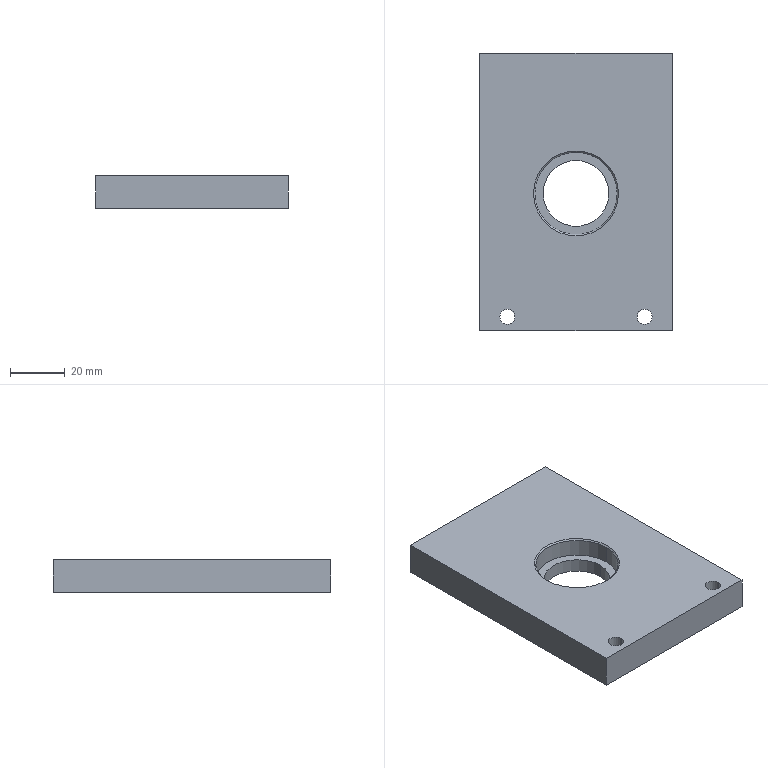Part | SolidWorks | features ICE 3, Chamfer 1, Extrusion 1, HoleWzd 1 | 1 solid | 25 faces | box 70 x 101 x 12 mm | volume 76361 mm3 | cylinder 12 | plane 7 | cone 6 | commonest cylinder face diameters 5 x4 5.5 x4 24 x2 30 x2
STEP:
#1=CARTESIAN_POINT('',(12.75,-96.,12.));
#2=VERTEX_POINT('',#1);
#3=CARTESIAN_POINT('',(7.25,-96.,12.));
#4=VERTEX_POINT('',#3);
#5=CARTESIAN_POINT('',(10.,-96.,12.));
#6=DIRECTION('',(0.,0.,-1.));
#7=DIRECTION('',(-1.,0.,0.));
#8=AXIS2_PLACEMENT_3D('',#5,#6,#7);
#9=CIRCLE('',#8,2.75);
#10=EDGE_CURVE('',#2,#4,#9,.T.);
#11=ORIENTED_EDGE('',*,*,#10,.F.);
#12=CARTESIAN_POINT('',(12.75,-96.,0.));
#13=VERTEX_POINT('',#12);
#14=CARTESIAN_POINT('',(12.75,-96.,12.));
#15=DIRECTION('',(0.,0.,-1.));
#16=VECTOR('',#15,1000.);
#17=LINE('',#14,#16);
#18=EDGE_CURVE('',#2,#13,#17,.T.);
#19=ORIENTED_EDGE('',*,*,#18,.T.);
#20=CARTESIAN_POINT('',(7.25,-96.,0.));
#21=VERTEX_POINT('',#20);
#22=CARTESIAN_POINT('',(10.,-96.,0.));
#23=DIRECTION('',(0.,0.,-1.));
#24=DIRECTION('',(-1.,0.,0.));
#25=AXIS2_PLACEMENT_3D('',#22,#23,#24);
#26=CIRCLE('',#25,2.75);
#27=EDGE_CURVE('',#13,#21,#26,.T.);
#28=ORIENTED_EDGE('',*,*,#27,.T.);
#29=CARTESIAN_POINT('',(7.25,-96.,12.));
#30=DIRECTION('',(0.,0.,-1.));
#31=VECTOR('',#30,1000.);
#32=LINE('',#29,#31);
#33=EDGE_CURVE('',#4,#21,#32,.T.);
#34=ORIENTED_EDGE('',*,*,#33,.F.);
#35=EDGE_LOOP('',(#11,#19,#28,#34));
#36=FACE_OUTER_BOUND('',#35,.T.);
#37=CARTESIAN_POINT('',(10.,-96.,12.));
#38=DIRECTION('',(0.,0.,-1.));
#39=DIRECTION('',(-1.,0.,0.));
#40=AXIS2_PLACEMENT_3D('',#37,#38,#39);
#41=CYLINDRICAL_SURFACE('',#40,2.75);
#42=ADVANCED_FACE('',(#36),#41,.F.);
#43=CARTESIAN_POINT('',(62.75,-96.,12.));
#44=VERTEX_POINT('',#43);
#45=CARTESIAN_POINT('',(57.25,-96.,12.));
#46=VERTEX_POINT('',#45);
#47=CARTESIAN_POINT('',(60.,-96.,12.));
#48=DIRECTION('',(0.,0.,-1.));
#49=DIRECTION('',(-1.,0.,0.));
#50=AXIS2_PLACEMENT_3D('',#47,#48,#49);
#51=CIRCLE('',#50,2.75);
#52=EDGE_CURVE('',#44,#46,#51,.T.);
#53=ORIENTED_EDGE('',*,*,#52,.F.);
#54=CARTESIAN_POINT('',(62.75,-96.,0.));
#55=VERTEX_POINT('',#54);
#56=CARTESIAN_POINT('',(62.75,-96.,12.));
#57=DIRECTION('',(0.,0.,-1.));
#58=VECTOR('',#57,1000.);
#59=LINE('',#56,#58);
#60=EDGE_CURVE('',#44,#55,#59,.T.);
#61=ORIENTED_EDGE('',*,*,#60,.T.);
#62=CARTESIAN_POINT('',(57.25,-96.,0.));
#63=VERTEX_POINT('',#62);
#64=CARTESIAN_POINT('',(60.,-96.,0.));
#65=DIRECTION('',(0.,0.,-1.));
#66=DIRECTION('',(-1.,0.,0.));
#67=AXIS2_PLACEMENT_3D('',#64,#65,#66);
#68=CIRCLE('',#67,2.75);
#69=EDGE_CURVE('',#55,#63,#68,.T.);
#70=ORIENTED_EDGE('',*,*,#69,.T.);
#71=CARTESIAN_POINT('',(57.25,-96.,12.));
#72=DIRECTION('',(0.,0.,-1.));
#73=VECTOR('',#72,1000.);
#74=LINE('',#71,#73);
#75=EDGE_CURVE('',#46,#63,#74,.T.);
#76=ORIENTED_EDGE('',*,*,#75,.F.);
#77=EDGE_LOOP('',(#53,#61,#70,#76));
#78=FACE_OUTER_BOUND('',#77,.T.);
#79=CARTESIAN_POINT('',(60.,-96.,12.));
#80=DIRECTION('',(0.,0.,-1.));
#81=DIRECTION('',(-1.,0.,0.));
#82=AXIS2_PLACEMENT_3D('',#79,#80,#81);
#83=CYLINDRICAL_SURFACE('',#82,2.75);
#84=ADVANCED_FACE('',(#78),#83,.F.);
#85=CARTESIAN_POINT('',(62.5,-17.,3.5));
#86=VERTEX_POINT('',#85);
#87=CARTESIAN_POINT('',(62.5,-17.,8.5));
#88=VERTEX_POINT('',#87);
#89=CARTESIAN_POINT('',(62.5,-17.,6.));
#90=DIRECTION('',(0.,1.,0.));
#91=DIRECTION('',(0.,0.,1.));
#92=AXIS2_PLACEMENT_3D('',#89,#90,#91);
#93=CIRCLE('',#92,2.5);
#94=EDGE_CURVE('',#86,#88,#93,.T.);
#95=ORIENTED_EDGE('',*,*,#94,.F.);
#96=CARTESIAN_POINT('',(62.5,0.,3.5));
#97=VERTEX_POINT('',#96);
#98=CARTESIAN_POINT('',(62.5,0.,3.5));
#99=DIRECTION('',(0.,1.,0.));
#100=VECTOR('',#99,1000.);
#101=LINE('',#98,#100);
#102=EDGE_CURVE('',#86,#97,#101,.T.);
#103=ORIENTED_EDGE('',*,*,#102,.T.);
#104=CARTESIAN_POINT('',(62.5,0.,8.5));
#105=VERTEX_POINT('',#104);
#106=CARTESIAN_POINT('',(62.5,0.,6.));
#107=DIRECTION('',(0.,1.,0.));
#108=DIRECTION('',(0.,0.,1.));
#109=AXIS2_PLACEMENT_3D('',#106,#107,#108);
#110=CIRCLE('',#109,2.5);
#111=EDGE_CURVE('',#97,#105,#110,.T.);
#112=ORIENTED_EDGE('',*,*,#111,.T.);
#113=CARTESIAN_POINT('',(62.5,0.,8.5));
#114=DIRECTION('',(0.,1.,0.));
#115=VECTOR('',#114,1000.);
#116=LINE('',#113,#115);
#117=EDGE_CURVE('',#88,#105,#116,.T.);
#118=ORIENTED_EDGE('',*,*,#117,.F.);
#119=EDGE_LOOP('',(#95,#103,#112,#118));
#120=FACE_OUTER_BOUND('',#119,.T.);
#121=CARTESIAN_POINT('',(62.5,0.,6.));
#122=DIRECTION('',(0.,1.,0.));
#123=DIRECTION('',(0.,0.,1.));
#124=AXIS2_PLACEMENT_3D('',#121,#122,#123);
#125=CYLINDRICAL_SURFACE('',#124,2.5);
#126=ADVANCED_FACE('',(#120),#125,.F.);
#127=CARTESIAN_POINT('',(62.5,-18.502,6.));
#128=VERTEX_POINT('',#127);
#129=CARTESIAN_POINT('',(62.5,-17.,8.5));
#130=DIRECTION('',(0.,0.515,0.8572));
#131=VECTOR('',#130,1000.);
#132=LINE('',#129,#131);
#133=EDGE_CURVE('',#128,#88,#132,.T.);
#134=ORIENTED_EDGE('',*,*,#133,.F.);
#135=CARTESIAN_POINT('',(62.5,-17.,3.5));
#136=DIRECTION('',(0.,0.515,-0.8572));
#137=VECTOR('',#136,1000.);
#138=LINE('',#135,#137);
#139=EDGE_CURVE('',#128,#86,#138,.T.);
#140=ORIENTED_EDGE('',*,*,#139,.T.);
#141=ORIENTED_EDGE('',*,*,#94,.T.);
#142=EDGE_LOOP('',(#134,#140,#141));
#143=FACE_OUTER_BOUND('',#142,.T.);
#144=CARTESIAN_POINT('',(62.5,-17.,6.));
#145=DIRECTION('',(0.,1.,0.));
#146=DIRECTION('',(0.,0.,1.));
#147=AXIS2_PLACEMENT_3D('',#144,#145,#146);
#148=CONICAL_SURFACE('',#147,2.5,1.03);
#149=ADVANCED_FACE('',(#143),#148,.F.);
#150=CARTESIAN_POINT('',(7.5,-17.,3.5));
#151=VERTEX_POINT('',#150);
#152=CARTESIAN_POINT('',(7.5,-17.,8.5));
#153=VERTEX_POINT('',#152);
#154=CARTESIAN_POINT('',(7.5,-17.,6.));
#155=DIRECTION('',(0.,1.,0.));
#156=DIRECTION('',(0.,0.,1.));
#157=AXIS2_PLACEMENT_3D('',#154,#155,#156);
#158=CIRCLE('',#157,2.5);
#159=EDGE_CURVE('',#151,#153,#158,.T.);
#160=ORIENTED_EDGE('',*,*,#159,.F.);
#161=CARTESIAN_POINT('',(7.5,0.,3.5));
#162=VERTEX_POINT('',#161);
#163=CARTESIAN_POINT('',(7.5,0.,3.5));
#164=DIRECTION('',(0.,1.,0.));
#165=VECTOR('',#164,1000.);
#166=LINE('',#163,#165);
#167=EDGE_CURVE('',#151,#162,#166,.T.);
#168=ORIENTED_EDGE('',*,*,#167,.T.);
#169=CARTESIAN_POINT('',(7.5,0.,8.5));
#170=VERTEX_POINT('',#169);
#171=CARTESIAN_POINT('',(7.5,0.,6.));
#172=DIRECTION('',(0.,1.,0.));
#173=DIRECTION('',(0.,0.,1.));
#174=AXIS2_PLACEMENT_3D('',#171,#172,#173);
#175=CIRCLE('',#174,2.5);
#176=EDGE_CURVE('',#162,#170,#175,.T.);
#177=ORIENTED_EDGE('',*,*,#176,.T.);
#178=CARTESIAN_POINT('',(7.5,0.,8.5));
#179=DIRECTION('',(0.,1.,0.));
#180=VECTOR('',#179,1000.);
#181=LINE('',#178,#180);
#182=EDGE_CURVE('',#153,#170,#181,.T.);
#183=ORIENTED_EDGE('',*,*,#182,.F.);
#184=EDGE_LOOP('',(#160,#168,#177,#183));
#185=FACE_OUTER_BOUND('',#184,.T.);
#186=CARTESIAN_POINT('',(7.5,0.,6.));
#187=DIRECTION('',(0.,1.,0.));
#188=DIRECTION('',(0.,0.,1.));
#189=AXIS2_PLACEMENT_3D('',#186,#187,#188);
#190=CYLINDRICAL_SURFACE('',#189,2.5);
#191=ADVANCED_FACE('',(#185),#190,.F.);
#192=CARTESIAN_POINT('',(7.5,-18.502,6.));
#193=VERTEX_POINT('',#192);
#194=CARTESIAN_POINT('',(7.5,-17.,8.5));
#195=DIRECTION('',(0.,0.515,0.8572));
#196=VECTOR('',#195,1000.);
#197=LINE('',#194,#196);
#198=EDGE_CURVE('',#193,#153,#197,.T.);
#199=ORIENTED_EDGE('',*,*,#198,.F.);
#200=CARTESIAN_POINT('',(7.5,-17.,3.5));
#201=DIRECTION('',(0.,0.515,-0.8572));
#202=VECTOR('',#201,1000.);
#203=LINE('',#200,#202);
#204=EDGE_CURVE('',#193,#151,#203,.T.);
#205=ORIENTED_EDGE('',*,*,#204,.T.);
#206=ORIENTED_EDGE('',*,*,#159,.T.);
#207=EDGE_LOOP('',(#199,#205,#206));
#208=FACE_OUTER_BOUND('',#207,.T.);
#209=CARTESIAN_POINT('',(7.5,-17.,6.));
#210=DIRECTION('',(0.,1.,0.));
#211=DIRECTION('',(0.,0.,1.));
#212=AXIS2_PLACEMENT_3D('',#209,#210,#211);
#213=CONICAL_SURFACE('',#212,2.5,1.03);
#214=ADVANCED_FACE('',(#208),#213,.F.);
#215=CARTESIAN_POINT('',(20.,-51.,11.5));
#216=VERTEX_POINT('',#215);
#217=CARTESIAN_POINT('',(50.,-51.,11.5));
#218=VERTEX_POINT('',#217);
#219=CARTESIAN_POINT('',(35.,-51.,11.5));
#220=DIRECTION('',(0.,0.,1.));
#221=DIRECTION('',(1.,0.,0.));
#222=AXIS2_PLACEMENT_3D('',#219,#220,#221);
#223=CIRCLE('',#222,15.);
#224=EDGE_CURVE('',#216,#218,#223,.T.);
#225=ORIENTED_EDGE('',*,*,#224,.F.);
#226=CARTESIAN_POINT('',(19.5,-51.,12.));
#227=VERTEX_POINT('',#226);
#228=CARTESIAN_POINT('',(20.,-51.,11.5));
#229=DIRECTION('',(-0.7071,0.,0.7071));
#230=VECTOR('',#229,1000.);
#231=LINE('',#228,#230);
#232=EDGE_CURVE('',#216,#227,#231,.T.);
#233=ORIENTED_EDGE('',*,*,#232,.T.);
#234=CARTESIAN_POINT('',(50.5,-51.,12.));
#235=VERTEX_POINT('',#234);
#236=CARTESIAN_POINT('',(35.,-51.,12.));
#237=DIRECTION('',(0.,0.,-1.));
#238=DIRECTION('',(1.,0.,0.));
#239=AXIS2_PLACEMENT_3D('',#236,#237,#238);
#240=CIRCLE('',#239,15.5);
#241=EDGE_CURVE('',#235,#227,#240,.T.);
#242=ORIENTED_EDGE('',*,*,#241,.F.);
#243=CARTESIAN_POINT('',(50.,-51.,11.5));
#244=DIRECTION('',(0.7071,0.,0.7071));
#245=VECTOR('',#244,1000.);
#246=LINE('',#243,#245);
#247=EDGE_CURVE('',#218,#235,#246,.T.);
#248=ORIENTED_EDGE('',*,*,#247,.F.);
#249=EDGE_LOOP('',(#225,#233,#242,#248));
#250=FACE_OUTER_BOUND('',#249,.T.);
#251=CARTESIAN_POINT('',(35.,-51.,11.5));
#252=DIRECTION('',(0.,0.,1.));
#253=DIRECTION('',(1.,0.,0.));
#254=AXIS2_PLACEMENT_3D('',#251,#252,#253);
#255=CONICAL_SURFACE('',#254,15.,0.7854);
#256=ADVANCED_FACE('',(#250),#255,.F.);
#257=CARTESIAN_POINT('',(23.,-51.,0.));
#258=VERTEX_POINT('',#257);
#259=CARTESIAN_POINT('',(47.,-51.,0.));
#260=VERTEX_POINT('',#259);
#261=CARTESIAN_POINT('',(35.,-51.,0.));
#262=DIRECTION('',(0.,0.,1.));
#263=DIRECTION('',(1.,0.,0.));
#264=AXIS2_PLACEMENT_3D('',#261,#262,#263);
#265=CIRCLE('',#264,12.);
#266=EDGE_CURVE('',#258,#260,#265,.T.);
#267=ORIENTED_EDGE('',*,*,#266,.F.);
#268=CARTESIAN_POINT('',(23.,-51.,5.));
#269=VERTEX_POINT('',#268);
#270=CARTESIAN_POINT('',(23.,-51.,0.));
#271=DIRECTION('',(0.,0.,1.));
#272=VECTOR('',#271,1000.);
#273=LINE('',#270,#272);
#274=EDGE_CURVE('',#258,#269,#273,.T.);
#275=ORIENTED_EDGE('',*,*,#274,.T.);
#276=CARTESIAN_POINT('',(47.,-51.,5.));
#277=VERTEX_POINT('',#276);
#278=CARTESIAN_POINT('',(35.,-51.,5.));
#279=DIRECTION('',(0.,0.,1.));
#280=DIRECTION('',(1.,0.,0.));
#281=AXIS2_PLACEMENT_3D('',#278,#279,#280);
#282=CIRCLE('',#281,12.);
#283=EDGE_CURVE('',#269,#277,#282,.T.);
#284=ORIENTED_EDGE('',*,*,#283,.T.);
#285=CARTESIAN_POINT('',(47.,-51.,0.));
#286=DIRECTION('',(0.,0.,1.));
#287=VECTOR('',#286,1000.);
#288=LINE('',#285,#287);
#289=EDGE_CURVE('',#260,#277,#288,.T.);
#290=ORIENTED_EDGE('',*,*,#289,.F.);
#291=EDGE_LOOP('',(#267,#275,#284,#290));
#292=FACE_OUTER_BOUND('',#291,.T.);
#293=CARTESIAN_POINT('',(35.,-51.,0.));
#294=DIRECTION('',(0.,0.,1.));
#295=DIRECTION('',(1.,0.,0.));
#296=AXIS2_PLACEMENT_3D('',#293,#294,#295);
#297=CYLINDRICAL_SURFACE('',#296,12.);
#298=ADVANCED_FACE('',(#292),#297,.F.);
#299=CARTESIAN_POINT('',(20.,-51.,5.));
#300=VERTEX_POINT('',#299);
#301=CARTESIAN_POINT('',(50.,-51.,5.));
#302=VERTEX_POINT('',#301);
#303=CARTESIAN_POINT('',(35.,-51.,5.));
#304=DIRECTION('',(0.,0.,1.));
#305=DIRECTION('',(1.,0.,0.));
#306=AXIS2_PLACEMENT_3D('',#303,#304,#305);
#307=CIRCLE('',#306,15.);
#308=EDGE_CURVE('',#300,#302,#307,.T.);
#309=ORIENTED_EDGE('',*,*,#308,.F.);
#310=CARTESIAN_POINT('',(20.,-51.,5.));
#311=DIRECTION('',(0.,0.,1.));
#312=VECTOR('',#311,1000.);
#313=LINE('',#310,#312);
#314=EDGE_CURVE('',#300,#216,#313,.T.);
#315=ORIENTED_EDGE('',*,*,#314,.T.);
#316=ORIENTED_EDGE('',*,*,#224,.T.);
#317=CARTESIAN_POINT('',(50.,-51.,5.));
#318=DIRECTION('',(0.,0.,1.));
#319=VECTOR('',#318,1000.);
#320=LINE('',#317,#319);
#321=EDGE_CURVE('',#302,#218,#320,.T.);
#322=ORIENTED_EDGE('',*,*,#321,.F.);
#323=EDGE_LOOP('',(#309,#315,#316,#322));
#324=FACE_OUTER_BOUND('',#323,.T.);
#325=CARTESIAN_POINT('',(35.,-51.,5.));
#326=DIRECTION('',(0.,0.,1.));
#327=DIRECTION('',(1.,0.,0.));
#328=AXIS2_PLACEMENT_3D('',#325,#326,#327);
#329=CYLINDRICAL_SURFACE('',#328,15.);
#330=ADVANCED_FACE('',(#324),#329,.F.);
#331=CARTESIAN_POINT('',(0.,0.,0.));
#332=VERTEX_POINT('',#331);
#333=CARTESIAN_POINT('',(0.,-101.,0.));
#334=VERTEX_POINT('',#333);
#335=CARTESIAN_POINT('',(0.,0.,0.));
#336=DIRECTION('',(0.,-1.,0.));
#337=VECTOR('',#336,1000.);
#338=LINE('',#335,#337);
#339=EDGE_CURVE('',#332,#334,#338,.T.);
#340=ORIENTED_EDGE('',*,*,#339,.T.);
#341=CARTESIAN_POINT('',(0.,-101.,12.));
#342=VERTEX_POINT('',#341);
#343=CARTESIAN_POINT('',(0.,-101.,12.));
#344=DIRECTION('',(0.,0.,-1.));
#345=VECTOR('',#344,1000.);
#346=LINE('',#343,#345);
#347=EDGE_CURVE('',#342,#334,#346,.T.);
#348=ORIENTED_EDGE('',*,*,#347,.F.);
#349=CARTESIAN_POINT('',(0.,0.,12.));
#350=VERTEX_POINT('',#349);
#351=CARTESIAN_POINT('',(0.,0.,12.));
#352=DIRECTION('',(0.,-1.,0.));
#353=VECTOR('',#352,1000.);
#354=LINE('',#351,#353);
#355=EDGE_CURVE('',#350,#342,#354,.T.);
#356=ORIENTED_EDGE('',*,*,#355,.F.);
#357=CARTESIAN_POINT('',(0.,0.,12.));
#358=DIRECTION('',(0.,0.,-1.));
#359=VECTOR('',#358,1000.);
#360=LINE('',#357,#359);
#361=EDGE_CURVE('',#350,#332,#360,.T.);
#362=ORIENTED_EDGE('',*,*,#361,.T.);
#363=EDGE_LOOP('',(#340,#348,#356,#362));
#364=FACE_OUTER_BOUND('',#363,.T.);
#365=CARTESIAN_POINT('',(0.,0.,12.));
#366=DIRECTION('',(1.,0.,0.));
#367=DIRECTION('',(0.,1.,0.));
#368=AXIS2_PLACEMENT_3D('',#365,#366,#367);
#369=PLANE('',#368);
#370=ADVANCED_FACE('',(#364),#369,.F.);
#371=CARTESIAN_POINT('',(70.,-101.,0.));
#372=VERTEX_POINT('',#371);
#373=CARTESIAN_POINT('',(0.,-101.,0.));
#374=DIRECTION('',(1.,0.,0.));
#375=VECTOR('',#374,1000.);
#376=LINE('',#373,#375);
#377=EDGE_CURVE('',#334,#372,#376,.T.);
#378=ORIENTED_EDGE('',*,*,#377,.T.);
#379=CARTESIAN_POINT('',(70.,-101.,12.));
#380=VERTEX_POINT('',#379);
#381=CARTESIAN_POINT('',(70.,-101.,12.));
#382=DIRECTION('',(0.,0.,-1.));
#383=VECTOR('',#382,1000.);
#384=LINE('',#381,#383);
#385=EDGE_CURVE('',#380,#372,#384,.T.);
#386=ORIENTED_EDGE('',*,*,#385,.F.);
#387=CARTESIAN_POINT('',(0.,-101.,12.));
#388=DIRECTION('',(1.,0.,0.));
#389=VECTOR('',#388,1000.);
#390=LINE('',#387,#389);
#391=EDGE_CURVE('',#342,#380,#390,.T.);
#392=ORIENTED_EDGE('',*,*,#391,.F.);
#393=ORIENTED_EDGE('',*,*,#347,.T.);
#394=EDGE_LOOP('',(#378,#386,#392,#393));
#395=FACE_OUTER_BOUND('',#394,.T.);
#396=CARTESIAN_POINT('',(0.,-101.,12.));
#397=DIRECTION('',(0.,1.,0.));
#398=DIRECTION('',(0.,0.,1.));
#399=AXIS2_PLACEMENT_3D('',#396,#397,#398);
#400=PLANE('',#399);
#401=ADVANCED_FACE('',(#395),#400,.F.);
#402=CARTESIAN_POINT('',(70.,0.,0.));
#403=VERTEX_POINT('',#402);
#404=CARTESIAN_POINT('',(70.,0.,0.));
#405=DIRECTION('',(0.,1.,0.));
#406=VECTOR('',#405,1000.);
#407=LINE('',#404,#406);
#408=EDGE_CURVE('',#372,#403,#407,.T.);
#409=ORIENTED_EDGE('',*,*,#408,.T.);
#410=CARTESIAN_POINT('',(70.,0.,12.));
#411=VERTEX_POINT('',#410);
#412=CARTESIAN_POINT('',(70.,0.,12.));
#413=DIRECTION('',(0.,0.,-1.));
#414=VECTOR('',#413,1000.);
#415=LINE('',#412,#414);
#416=EDGE_CURVE('',#411,#403,#415,.T.);
#417=ORIENTED_EDGE('',*,*,#416,.F.);
#418=CARTESIAN_POINT('',(70.,0.,12.));
#419=DIRECTION('',(0.,1.,0.));
#420=VECTOR('',#419,1000.);
#421=LINE('',#418,#420);
#422=EDGE_CURVE('',#380,#411,#421,.T.);
#423=ORIENTED_EDGE('',*,*,#422,.F.);
#424=ORIENTED_EDGE('',*,*,#385,.T.);
#425=EDGE_LOOP('',(#409,#417,#423,#424));
#426=FACE_OUTER_BOUND('',#425,.T.);
#427=CARTESIAN_POINT('',(70.,0.,12.));
#428=DIRECTION('',(-1.,0.,0.));
#429=DIRECTION('',(0.,0.,1.));
#430=AXIS2_PLACEMENT_3D('',#427,#428,#429);
#431=PLANE('',#430);
#432=ADVANCED_FACE('',(#426),#431,.F.);
#433=CARTESIAN_POINT('',(62.5,0.,6.));
#434=DIRECTION('',(0.,1.,0.));
#435=DIRECTION('',(0.,0.,1.));
#436=AXIS2_PLACEMENT_3D('',#433,#434,#435);
#437=CIRCLE('',#436,2.5);
#438=EDGE_CURVE('',#105,#97,#437,.T.);
#439=ORIENTED_EDGE('',*,*,#438,.F.);
#440=ORIENTED_EDGE('',*,*,#111,.F.);
#441=EDGE_LOOP('',(#439,#440));
#442=FACE_BOUND('',#441,.T.);
#443=CARTESIAN_POINT('',(7.5,0.,6.));
#444=DIRECTION('',(0.,1.,0.));
#445=DIRECTION('',(0.,0.,1.));
#446=AXIS2_PLACEMENT_3D('',#443,#444,#445);
#447=CIRCLE('',#446,2.5);
#448=EDGE_CURVE('',#170,#162,#447,.T.);
#449=ORIENTED_EDGE('',*,*,#448,.F.);
#450=ORIENTED_EDGE('',*,*,#176,.F.);
#451=EDGE_LOOP('',(#449,#450));
#452=FACE_BOUND('',#451,.T.);
#453=CARTESIAN_POINT('',(0.,0.,0.));
#454=DIRECTION('',(-1.,0.,0.));
#455=VECTOR('',#454,1000.);
#456=LINE('',#453,#455);
#457=EDGE_CURVE('',#403,#332,#456,.T.);
#458=ORIENTED_EDGE('',*,*,#457,.T.);
#459=ORIENTED_EDGE('',*,*,#361,.F.);
#460=CARTESIAN_POINT('',(0.,0.,12.));
#461=DIRECTION('',(-1.,0.,0.));
#462=VECTOR('',#461,1000.);
#463=LINE('',#460,#462);
#464=EDGE_CURVE('',#411,#350,#463,.T.);
#465=ORIENTED_EDGE('',*,*,#464,.F.);
#466=ORIENTED_EDGE('',*,*,#416,.T.);
#467=EDGE_LOOP('',(#458,#459,#465,#466));
#468=FACE_OUTER_BOUND('',#467,.T.);
#469=CARTESIAN_POINT('',(0.,0.,12.));
#470=DIRECTION('',(0.,-1.,0.));
#471=DIRECTION('',(0.,0.,-1.));
#472=AXIS2_PLACEMENT_3D('',#469,#470,#471);
#473=PLANE('',#472);
#474=ADVANCED_FACE('',(#442,#452,#468),#473,.F.);
#475=CARTESIAN_POINT('',(10.,-96.,12.));
#476=DIRECTION('',(0.,0.,-1.));
#477=DIRECTION('',(-1.,0.,0.));
#478=AXIS2_PLACEMENT_3D('',#475,#476,#477);
#479=CIRCLE('',#478,2.75);
#480=EDGE_CURVE('',#4,#2,#479,.T.);
#481=ORIENTED_EDGE('',*,*,#480,.T.);
#482=ORIENTED_EDGE('',*,*,#10,.T.);
#483=EDGE_LOOP('',(#481,#482));
#484=FACE_BOUND('',#483,.T.);
#485=CARTESIAN_POINT('',(60.,-96.,12.));
#486=DIRECTION('',(0.,0.,-1.));
#487=DIRECTION('',(-1.,0.,0.));
#488=AXIS2_PLACEMENT_3D('',#485,#486,#487);
#489=CIRCLE('',#488,2.75);
#490=EDGE_CURVE('',#46,#44,#489,.T.);
#491=ORIENTED_EDGE('',*,*,#490,.T.);
#492=ORIENTED_EDGE('',*,*,#52,.T.);
#493=EDGE_LOOP('',(#491,#492));
#494=FACE_BOUND('',#493,.T.);
#495=ORIENTED_EDGE('',*,*,#241,.T.);
#496=CARTESIAN_POINT('',(35.,-51.,12.));
#497=DIRECTION('',(0.,0.,-1.));
#498=DIRECTION('',(1.,0.,0.));
#499=AXIS2_PLACEMENT_3D('',#496,#497,#498);
#500=CIRCLE('',#499,15.5);
#501=EDGE_CURVE('',#227,#235,#500,.T.);
#502=ORIENTED_EDGE('',*,*,#501,.T.);
#503=EDGE_LOOP('',(#495,#502));
#504=FACE_BOUND('',#503,.T.);
#505=ORIENTED_EDGE('',*,*,#355,.T.);
#506=ORIENTED_EDGE('',*,*,#391,.T.);
#507=ORIENTED_EDGE('',*,*,#422,.T.);
#508=ORIENTED_EDGE('',*,*,#464,.T.);
#509=EDGE_LOOP('',(#505,#506,#507,#508));
#510=FACE_OUTER_BOUND('',#509,.T.);
#511=CARTESIAN_POINT('',(0.,0.,12.));
#512=DIRECTION('',(0.,0.,1.));
#513=DIRECTION('',(1.,0.,0.));
#514=AXIS2_PLACEMENT_3D('',#511,#512,#513);
#515=PLANE('',#514);
#516=ADVANCED_FACE('',(#484,#494,#504,#510),#515,.T.);
#517=CARTESIAN_POINT('',(10.,-96.,0.));
#518=DIRECTION('',(0.,0.,-1.));
#519=DIRECTION('',(-1.,0.,0.));
#520=AXIS2_PLACEMENT_3D('',#517,#518,#519);
#521=CIRCLE('',#520,2.75);
#522=EDGE_CURVE('',#21,#13,#521,.T.);
#523=ORIENTED_EDGE('',*,*,#522,.F.);
#524=ORIENTED_EDGE('',*,*,#27,.F.);
#525=EDGE_LOOP('',(#523,#524));
#526=FACE_BOUND('',#525,.T.);
#527=CARTESIAN_POINT('',(60.,-96.,0.));
#528=DIRECTION('',(0.,0.,-1.));
#529=DIRECTION('',(-1.,0.,0.));
#530=AXIS2_PLACEMENT_3D('',#527,#528,#529);
#531=CIRCLE('',#530,2.75);
#532=EDGE_CURVE('',#63,#55,#531,.T.);
#533=ORIENTED_EDGE('',*,*,#532,.F.);
#534=ORIENTED_EDGE('',*,*,#69,.F.);
#535=EDGE_LOOP('',(#533,#534));
#536=FACE_BOUND('',#535,.T.);
#537=CARTESIAN_POINT('',(35.,-51.,0.));
#538=DIRECTION('',(0.,0.,1.));
#539=DIRECTION('',(1.,0.,0.));
#540=AXIS2_PLACEMENT_3D('',#537,#538,#539);
#541=CIRCLE('',#540,12.);
#542=EDGE_CURVE('',#260,#258,#541,.T.);
#543=ORIENTED_EDGE('',*,*,#542,.T.);
#544=ORIENTED_EDGE('',*,*,#266,.T.);
#545=EDGE_LOOP('',(#543,#544));
#546=FACE_BOUND('',#545,.T.);
#547=ORIENTED_EDGE('',*,*,#339,.F.);
#548=ORIENTED_EDGE('',*,*,#457,.F.);
#549=ORIENTED_EDGE('',*,*,#408,.F.);
#550=ORIENTED_EDGE('',*,*,#377,.F.);
#551=EDGE_LOOP('',(#547,#548,#549,#550));
#552=FACE_OUTER_BOUND('',#551,.T.);
#553=CARTESIAN_POINT('',(0.,0.,0.));
#554=DIRECTION('',(0.,0.,1.));
#555=DIRECTION('',(1.,0.,0.));
#556=AXIS2_PLACEMENT_3D('',#553,#554,#555);
#557=PLANE('',#556);
#558=ADVANCED_FACE('',(#526,#536,#546,#552),#557,.F.);
#559=ORIENTED_EDGE('',*,*,#314,.F.);
#560=CARTESIAN_POINT('',(35.,-51.,5.));
#561=DIRECTION('',(0.,0.,1.));
#562=DIRECTION('',(1.,0.,0.));
#563=AXIS2_PLACEMENT_3D('',#560,#561,#562);
#564=CIRCLE('',#563,15.);
#565=EDGE_CURVE('',#302,#300,#564,.T.);
#566=ORIENTED_EDGE('',*,*,#565,.F.);
#567=ORIENTED_EDGE('',*,*,#321,.T.);
#568=CARTESIAN_POINT('',(35.,-51.,11.5));
#569=DIRECTION('',(0.,0.,1.));
#570=DIRECTION('',(1.,0.,0.));
#571=AXIS2_PLACEMENT_3D('',#568,#569,#570);
#572=CIRCLE('',#571,15.);
#573=EDGE_CURVE('',#218,#216,#572,.T.);
#574=ORIENTED_EDGE('',*,*,#573,.T.);
#575=EDGE_LOOP('',(#559,#566,#567,#574));
#576=FACE_OUTER_BOUND('',#575,.T.);
#577=CARTESIAN_POINT('',(35.,-51.,5.));
#578=DIRECTION('',(0.,0.,1.));
#579=DIRECTION('',(1.,0.,0.));
#580=AXIS2_PLACEMENT_3D('',#577,#578,#579);
#581=CYLINDRICAL_SURFACE('',#580,15.);
#582=ADVANCED_FACE('',(#576),#581,.F.);
#583=CARTESIAN_POINT('',(35.,-51.,5.));
#584=DIRECTION('',(0.,0.,1.));
#585=DIRECTION('',(1.,0.,0.));
#586=AXIS2_PLACEMENT_3D('',#583,#584,#585);
#587=CIRCLE('',#586,12.);
#588=EDGE_CURVE('',#277,#269,#587,.T.);
#589=ORIENTED_EDGE('',*,*,#588,.F.);
#590=ORIENTED_EDGE('',*,*,#283,.F.);
#591=EDGE_LOOP('',(#589,#590));
#592=FACE_BOUND('',#591,.T.);
#593=ORIENTED_EDGE('',*,*,#565,.T.);
#594=ORIENTED_EDGE('',*,*,#308,.T.);
#595=EDGE_LOOP('',(#593,#594));
#596=FACE_OUTER_BOUND('',#595,.T.);
#597=CARTESIAN_POINT('',(35.,-51.,5.));
#598=DIRECTION('',(0.,0.,1.));
#599=DIRECTION('',(1.,0.,0.));
#600=AXIS2_PLACEMENT_3D('',#597,#598,#599);
#601=PLANE('',#600);
#602=ADVANCED_FACE('',(#592,#596),#601,.T.);
#603=ORIENTED_EDGE('',*,*,#274,.F.);
#604=ORIENTED_EDGE('',*,*,#542,.F.);
#605=ORIENTED_EDGE('',*,*,#289,.T.);
#606=ORIENTED_EDGE('',*,*,#588,.T.);
#607=EDGE_LOOP('',(#603,#604,#605,#606));
#608=FACE_OUTER_BOUND('',#607,.T.);
#609=CARTESIAN_POINT('',(35.,-51.,0.));
#610=DIRECTION('',(0.,0.,1.));
#611=DIRECTION('',(1.,0.,0.));
#612=AXIS2_PLACEMENT_3D('',#609,#610,#611);
#613=CYLINDRICAL_SURFACE('',#612,12.);
#614=ADVANCED_FACE('',(#608),#613,.F.);
#615=ORIENTED_EDGE('',*,*,#232,.F.);
#616=ORIENTED_EDGE('',*,*,#573,.F.);
#617=ORIENTED_EDGE('',*,*,#247,.T.);
#618=ORIENTED_EDGE('',*,*,#501,.F.);
#619=EDGE_LOOP('',(#615,#616,#617,#618));
#620=FACE_OUTER_BOUND('',#619,.T.);
#621=CARTESIAN_POINT('',(35.,-51.,11.5));
#622=DIRECTION('',(0.,0.,1.));
#623=DIRECTION('',(1.,0.,0.));
#624=AXIS2_PLACEMENT_3D('',#621,#622,#623);
#625=CONICAL_SURFACE('',#624,15.,0.7854);
#626=ADVANCED_FACE('',(#620),#625,.F.);
#627=ORIENTED_EDGE('',*,*,#204,.F.);
#628=ORIENTED_EDGE('',*,*,#198,.T.);
#629=CARTESIAN_POINT('',(7.5,-17.,6.));
#630=DIRECTION('',(0.,1.,0.));
#631=DIRECTION('',(0.,0.,1.));
#632=AXIS2_PLACEMENT_3D('',#629,#630,#631);
#633=CIRCLE('',#632,2.5);
#634=EDGE_CURVE('',#153,#151,#633,.T.);
#635=ORIENTED_EDGE('',*,*,#634,.T.);
#636=EDGE_LOOP('',(#627,#628,#635));
#637=FACE_OUTER_BOUND('',#636,.T.);
#638=CARTESIAN_POINT('',(7.5,-17.,6.));
#639=DIRECTION('',(0.,1.,0.));
#640=DIRECTION('',(0.,0.,1.));
#641=AXIS2_PLACEMENT_3D('',#638,#639,#640);
#642=CONICAL_SURFACE('',#641,2.5,1.03);
#643=ADVANCED_FACE('',(#637),#642,.F.);
#644=ORIENTED_EDGE('',*,*,#167,.F.);
#645=ORIENTED_EDGE('',*,*,#634,.F.);
#646=ORIENTED_EDGE('',*,*,#182,.T.);
#647=ORIENTED_EDGE('',*,*,#448,.T.);
#648=EDGE_LOOP('',(#644,#645,#646,#647));
#649=FACE_OUTER_BOUND('',#648,.T.);
#650=CARTESIAN_POINT('',(7.5,0.,6.));
#651=DIRECTION('',(0.,1.,0.));
#652=DIRECTION('',(0.,0.,1.));
#653=AXIS2_PLACEMENT_3D('',#650,#651,#652);
#654=CYLINDRICAL_SURFACE('',#653,2.5);
#655=ADVANCED_FACE('',(#649),#654,.F.);
#656=ORIENTED_EDGE('',*,*,#139,.F.);
#657=ORIENTED_EDGE('',*,*,#133,.T.);
#658=CARTESIAN_POINT('',(62.5,-17.,6.));
#659=DIRECTION('',(0.,1.,0.));
#660=DIRECTION('',(0.,0.,1.));
#661=AXIS2_PLACEMENT_3D('',#658,#659,#660);
#662=CIRCLE('',#661,2.5);
#663=EDGE_CURVE('',#88,#86,#662,.T.);
#664=ORIENTED_EDGE('',*,*,#663,.T.);
#665=EDGE_LOOP('',(#656,#657,#664));
#666=FACE_OUTER_BOUND('',#665,.T.);
#667=CARTESIAN_POINT('',(62.5,-17.,6.));
#668=DIRECTION('',(0.,1.,0.));
#669=DIRECTION('',(0.,0.,1.));
#670=AXIS2_PLACEMENT_3D('',#667,#668,#669);
#671=CONICAL_SURFACE('',#670,2.5,1.03);
#672=ADVANCED_FACE('',(#666),#671,.F.);
#673=ORIENTED_EDGE('',*,*,#102,.F.);
#674=ORIENTED_EDGE('',*,*,#663,.F.);
#675=ORIENTED_EDGE('',*,*,#117,.T.);
#676=ORIENTED_EDGE('',*,*,#438,.T.);
#677=EDGE_LOOP('',(#673,#674,#675,#676));
#678=FACE_OUTER_BOUND('',#677,.T.);
#679=CARTESIAN_POINT('',(62.5,0.,6.));
#680=DIRECTION('',(0.,1.,0.));
#681=DIRECTION('',(0.,0.,1.));
#682=AXIS2_PLACEMENT_3D('',#679,#680,#681);
#683=CYLINDRICAL_SURFACE('',#682,2.5);
#684=ADVANCED_FACE('',(#678),#683,.F.);
#685=ORIENTED_EDGE('',*,*,#60,.F.);
#686=ORIENTED_EDGE('',*,*,#490,.F.);
#687=ORIENTED_EDGE('',*,*,#75,.T.);
#688=ORIENTED_EDGE('',*,*,#532,.T.);
#689=EDGE_LOOP('',(#685,#686,#687,#688));
#690=FACE_OUTER_BOUND('',#689,.T.);
#691=CARTESIAN_POINT('',(60.,-96.,12.));
#692=DIRECTION('',(0.,0.,-1.));
#693=DIRECTION('',(-1.,0.,0.));
#694=AXIS2_PLACEMENT_3D('',#691,#692,#693);
#695=CYLINDRICAL_SURFACE('',#694,2.75);
#696=ADVANCED_FACE('',(#690),#695,.F.);
#697=ORIENTED_EDGE('',*,*,#18,.F.);
#698=ORIENTED_EDGE('',*,*,#480,.F.);
#699=ORIENTED_EDGE('',*,*,#33,.T.);
#700=ORIENTED_EDGE('',*,*,#522,.T.);
#701=EDGE_LOOP('',(#697,#698,#699,#700));
#702=FACE_OUTER_BOUND('',#701,.T.);
#703=CARTESIAN_POINT('',(10.,-96.,12.));
#704=DIRECTION('',(0.,0.,-1.));
#705=DIRECTION('',(-1.,0.,0.));
#706=AXIS2_PLACEMENT_3D('',#703,#704,#705);
#707=CYLINDRICAL_SURFACE('',#706,2.75);
#708=ADVANCED_FACE('',(#702),#707,.F.);
#709=CLOSED_SHELL('',(#42,#84,#126,#149,#191,#214,#256,#298,#330,#370,#401,#432,#474,#516,#558,#582,#602,#614,#626,#643,#655,#672,#684,#696,#708));
#710=MANIFOLD_SOLID_BREP('',#709);
#711=CARTESIAN_POINT('',(0.,0.,0.));
#712=DIRECTION('',(0.,0.,1.));
#713=DIRECTION('',(1.,0.,0.));
#714=AXIS2_PLACEMENT_3D('',#711,#712,#713);
#715=(LENGTH_UNIT()NAMED_UNIT(*)SI_UNIT(.MILLI.,.METRE.));
#716=UNCERTAINTY_MEASURE_WITH_UNIT(LENGTH_MEASURE(0.00001),#715,'','');
#717=(NAMED_UNIT(*)PLANE_ANGLE_UNIT()SI_UNIT($,.RADIAN.));
#718=(NAMED_UNIT(*)SI_UNIT($,.STERADIAN.)SOLID_ANGLE_UNIT());
#719=(GEOMETRIC_REPRESENTATION_CONTEXT(3)GLOBAL_UNCERTAINTY_ASSIGNED_CONTEXT((#716))GLOBAL_UNIT_ASSIGNED_CONTEXT((#715,#717,#718))REPRESENTATION_CONTEXT('',''));
#720=ADVANCED_BREP_SHAPE_REPRESENTATION('',(#710,#714),#719);